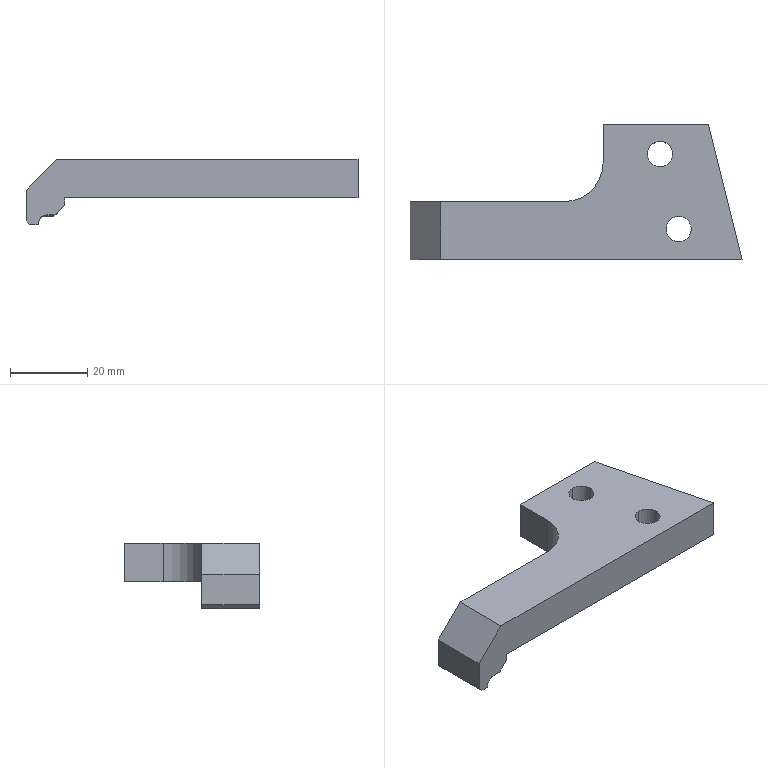Part | 1 solid | 24 faces | box 86 x 35 x 17 mm | volume 18400 mm3 | plane 13 | spline 6 | cylinder 5 | commonest cylinder face diameters 6.5 x4 20 x1
STEP:
#1=CARTESIAN_POINT('',(26.602,-12.85,-10.));
#2=VERTEX_POINT('',#1);
#3=CARTESIAN_POINT('',(26.602,-6.35,-10.));
#4=VERTEX_POINT('',#3);
#5=CARTESIAN_POINT('',(26.602,-9.6,-10.));
#6=DIRECTION('',(0.,0.,1.));
#7=DIRECTION('',(0.,1.,0.));
#8=AXIS2_PLACEMENT_3D('',#5,#6,#7);
#9=CIRCLE('',#8,3.25);
#10=EDGE_CURVE('',#2,#4,#9,.T.);
#11=ORIENTED_EDGE('',*,*,#10,.F.);
#12=CARTESIAN_POINT('',(26.602,-12.85,0.));
#13=VERTEX_POINT('',#12);
#14=CARTESIAN_POINT('',(26.602,-12.85,0.));
#15=DIRECTION('',(0.,0.,1.));
#16=VECTOR('',#15,1000.);
#17=LINE('',#14,#16);
#18=EDGE_CURVE('',#2,#13,#17,.T.);
#19=ORIENTED_EDGE('',*,*,#18,.T.);
#20=CARTESIAN_POINT('',(26.602,-6.35,0.));
#21=VERTEX_POINT('',#20);
#22=CARTESIAN_POINT('',(26.602,-9.6,0.));
#23=DIRECTION('',(0.,0.,1.));
#24=DIRECTION('',(0.,1.,0.));
#25=AXIS2_PLACEMENT_3D('',#22,#23,#24);
#26=CIRCLE('',#25,3.25);
#27=EDGE_CURVE('',#13,#21,#26,.T.);
#28=ORIENTED_EDGE('',*,*,#27,.T.);
#29=CARTESIAN_POINT('',(26.602,-6.35,0.));
#30=DIRECTION('',(0.,0.,1.));
#31=VECTOR('',#30,1000.);
#32=LINE('',#29,#31);
#33=EDGE_CURVE('',#4,#21,#32,.T.);
#34=ORIENTED_EDGE('',*,*,#33,.F.);
#35=EDGE_LOOP('',(#11,#19,#28,#34));
#36=FACE_BOUND('',#35,.T.);
#37=CARTESIAN_POINT('',(26.602,-9.6,0.));
#38=DIRECTION('',(0.,0.,1.));
#39=DIRECTION('',(0.,-1.,0.));
#40=AXIS2_PLACEMENT_3D('',#37,#38,#39);
#41=CYLINDRICAL_SURFACE('',#40,3.25);
#42=ADVANCED_FACE('',(#36),#41,.F.);
#43=CARTESIAN_POINT('',(21.763,6.556,-10.));
#44=VERTEX_POINT('',#43);
#45=CARTESIAN_POINT('',(21.763,13.056,-10.));
#46=VERTEX_POINT('',#45);
#47=CARTESIAN_POINT('',(21.763,9.806,-10.));
#48=DIRECTION('',(0.,0.,1.));
#49=DIRECTION('',(0.,1.,0.));
#50=AXIS2_PLACEMENT_3D('',#47,#48,#49);
#51=CIRCLE('',#50,3.25);
#52=EDGE_CURVE('',#44,#46,#51,.T.);
#53=ORIENTED_EDGE('',*,*,#52,.F.);
#54=CARTESIAN_POINT('',(21.763,6.556,0.));
#55=VERTEX_POINT('',#54);
#56=CARTESIAN_POINT('',(21.763,6.556,0.));
#57=DIRECTION('',(0.,0.,1.));
#58=VECTOR('',#57,1000.);
#59=LINE('',#56,#58);
#60=EDGE_CURVE('',#44,#55,#59,.T.);
#61=ORIENTED_EDGE('',*,*,#60,.T.);
#62=CARTESIAN_POINT('',(21.763,13.056,0.));
#63=VERTEX_POINT('',#62);
#64=CARTESIAN_POINT('',(21.763,9.806,0.));
#65=DIRECTION('',(0.,0.,1.));
#66=DIRECTION('',(0.,1.,0.));
#67=AXIS2_PLACEMENT_3D('',#64,#65,#66);
#68=CIRCLE('',#67,3.25);
#69=EDGE_CURVE('',#55,#63,#68,.T.);
#70=ORIENTED_EDGE('',*,*,#69,.T.);
#71=CARTESIAN_POINT('',(21.763,13.056,0.));
#72=DIRECTION('',(0.,0.,1.));
#73=VECTOR('',#72,1000.);
#74=LINE('',#71,#73);
#75=EDGE_CURVE('',#46,#63,#74,.T.);
#76=ORIENTED_EDGE('',*,*,#75,.F.);
#77=EDGE_LOOP('',(#53,#61,#70,#76));
#78=FACE_BOUND('',#77,.T.);
#79=CARTESIAN_POINT('',(21.763,9.806,0.));
#80=DIRECTION('',(0.,0.,1.));
#81=DIRECTION('',(0.,-1.,0.));
#82=AXIS2_PLACEMENT_3D('',#79,#80,#81);
#83=CYLINDRICAL_SURFACE('',#82,3.25);
#84=ADVANCED_FACE('',(#78),#83,.F.);
#85=CARTESIAN_POINT('',(21.763,9.806,0.));
#86=DIRECTION('',(0.,0.,1.));
#87=DIRECTION('',(0.,1.,0.));
#88=AXIS2_PLACEMENT_3D('',#85,#86,#87);
#89=CIRCLE('',#88,3.25);
#90=EDGE_CURVE('',#63,#55,#89,.T.);
#91=ORIENTED_EDGE('',*,*,#90,.F.);
#92=ORIENTED_EDGE('',*,*,#69,.F.);
#93=EDGE_LOOP('',(#91,#92));
#94=FACE_BOUND('',#93,.T.);
#95=CARTESIAN_POINT('',(26.602,-9.6,0.));
#96=DIRECTION('',(0.,0.,1.));
#97=DIRECTION('',(0.,1.,0.));
#98=AXIS2_PLACEMENT_3D('',#95,#96,#97);
#99=CIRCLE('',#98,3.25);
#100=EDGE_CURVE('',#21,#13,#99,.T.);
#101=ORIENTED_EDGE('',*,*,#100,.F.);
#102=ORIENTED_EDGE('',*,*,#27,.F.);
#103=EDGE_LOOP('',(#101,#102));
#104=FACE_BOUND('',#103,.T.);
#105=CARTESIAN_POINT('',(7.,17.5,0.));
#106=VERTEX_POINT('',#105);
#107=CARTESIAN_POINT('',(7.,7.5,0.));
#108=VERTEX_POINT('',#107);
#109=CARTESIAN_POINT('',(7.,17.5,0.));
#110=DIRECTION('',(0.,-1.,0.));
#111=VECTOR('',#110,1000.);
#112=LINE('',#109,#111);
#113=EDGE_CURVE('',#106,#108,#112,.T.);
#114=ORIENTED_EDGE('',*,*,#113,.T.);
#115=CARTESIAN_POINT('',(-3.,-2.5,0.));
#116=VERTEX_POINT('',#115);
#117=CARTESIAN_POINT('',(-3.,7.5,0.));
#118=DIRECTION('',(0.,0.,-1.));
#119=DIRECTION('',(-1.,0.,0.));
#120=AXIS2_PLACEMENT_3D('',#117,#118,#119);
#121=CIRCLE('',#120,10.);
#122=EDGE_CURVE('',#108,#116,#121,.T.);
#123=ORIENTED_EDGE('',*,*,#122,.T.);
#124=CARTESIAN_POINT('',(-35.,-2.5,0.));
#125=VERTEX_POINT('',#124);
#126=CARTESIAN_POINT('',(-43.,-2.5,0.));
#127=DIRECTION('',(1.,0.,0.));
#128=VECTOR('',#127,1000.);
#129=LINE('',#126,#128);
#130=EDGE_CURVE('',#125,#116,#129,.T.);
#131=ORIENTED_EDGE('',*,*,#130,.F.);
#132=CARTESIAN_POINT('',(-35.,-17.5,0.));
#133=VERTEX_POINT('',#132);
#134=CARTESIAN_POINT('',(-35.,17.5,0.));
#135=DIRECTION('',(0.,-1.,0.));
#136=VECTOR('',#135,1000.);
#137=LINE('',#134,#136);
#138=EDGE_CURVE('',#125,#133,#137,.T.);
#139=ORIENTED_EDGE('',*,*,#138,.T.);
#140=CARTESIAN_POINT('',(43.,-17.5,0.));
#141=VERTEX_POINT('',#140);
#142=CARTESIAN_POINT('',(-43.,-17.5,0.));
#143=DIRECTION('',(1.,0.,0.));
#144=VECTOR('',#143,1000.);
#145=LINE('',#142,#144);
#146=EDGE_CURVE('',#133,#141,#145,.T.);
#147=ORIENTED_EDGE('',*,*,#146,.T.);
#148=CARTESIAN_POINT('',(34.274,17.5,0.));
#149=VERTEX_POINT('',#148);
#150=CARTESIAN_POINT('',(34.274,17.5,0.));
#151=DIRECTION('',(0.2419,-0.9703,0.));
#152=VECTOR('',#151,1000.);
#153=LINE('',#150,#152);
#154=EDGE_CURVE('',#149,#141,#153,.T.);
#155=ORIENTED_EDGE('',*,*,#154,.F.);
#156=CARTESIAN_POINT('',(-43.,17.5,0.));
#157=DIRECTION('',(1.,0.,0.));
#158=VECTOR('',#157,1000.);
#159=LINE('',#156,#158);
#160=EDGE_CURVE('',#106,#149,#159,.T.);
#161=ORIENTED_EDGE('',*,*,#160,.F.);
#162=EDGE_LOOP('',(#114,#123,#131,#139,#147,#155,#161));
#163=FACE_BOUND('',#162,.T.);
#164=CARTESIAN_POINT('',(-43.,17.5,0.));
#165=DIRECTION('',(0.,0.,-1.));
#166=DIRECTION('',(1.,0.,0.));
#167=AXIS2_PLACEMENT_3D('',#164,#165,#166);
#168=PLANE('',#167);
#169=ADVANCED_FACE('',(#94,#104,#163),#168,.F.);
#170=CARTESIAN_POINT('',(21.763,9.806,-10.));
#171=DIRECTION('',(0.,0.,1.));
#172=DIRECTION('',(0.,1.,0.));
#173=AXIS2_PLACEMENT_3D('',#170,#171,#172);
#174=CIRCLE('',#173,3.25);
#175=EDGE_CURVE('',#46,#44,#174,.T.);
#176=ORIENTED_EDGE('',*,*,#175,.T.);
#177=ORIENTED_EDGE('',*,*,#52,.T.);
#178=EDGE_LOOP('',(#176,#177));
#179=FACE_BOUND('',#178,.T.);
#180=CARTESIAN_POINT('',(26.602,-9.6,-10.));
#181=DIRECTION('',(0.,0.,1.));
#182=DIRECTION('',(0.,1.,0.));
#183=AXIS2_PLACEMENT_3D('',#180,#181,#182);
#184=CIRCLE('',#183,3.25);
#185=EDGE_CURVE('',#4,#2,#184,.T.);
#186=ORIENTED_EDGE('',*,*,#185,.T.);
#187=ORIENTED_EDGE('',*,*,#10,.T.);
#188=EDGE_LOOP('',(#186,#187));
#189=FACE_BOUND('',#188,.T.);
#190=CARTESIAN_POINT('',(7.,17.5,-10.));
#191=VERTEX_POINT('',#190);
#192=CARTESIAN_POINT('',(7.,7.5,-10.));
#193=VERTEX_POINT('',#192);
#194=CARTESIAN_POINT('',(7.,17.5,-10.));
#195=DIRECTION('',(0.,-1.,0.));
#196=VECTOR('',#195,1000.);
#197=LINE('',#194,#196);
#198=EDGE_CURVE('',#191,#193,#197,.T.);
#199=ORIENTED_EDGE('',*,*,#198,.F.);
#200=CARTESIAN_POINT('',(34.274,17.5,-10.));
#201=VERTEX_POINT('',#200);
#202=CARTESIAN_POINT('',(43.,17.5,-10.));
#203=DIRECTION('',(-1.,0.,0.));
#204=VECTOR('',#203,1000.);
#205=LINE('',#202,#204);
#206=EDGE_CURVE('',#201,#191,#205,.T.);
#207=ORIENTED_EDGE('',*,*,#206,.F.);
#208=CARTESIAN_POINT('',(43.,-17.5,-10.));
#209=VERTEX_POINT('',#208);
#210=CARTESIAN_POINT('',(34.274,17.5,-10.));
#211=DIRECTION('',(-0.2419,0.9703,0.));
#212=VECTOR('',#211,1000.);
#213=LINE('',#210,#212);
#214=EDGE_CURVE('',#209,#201,#213,.T.);
#215=ORIENTED_EDGE('',*,*,#214,.F.);
#216=CARTESIAN_POINT('',(-33.,-17.5,-10.));
#217=VERTEX_POINT('',#216);
#218=CARTESIAN_POINT('',(43.,-17.5,-10.));
#219=DIRECTION('',(-1.,0.,0.));
#220=VECTOR('',#219,1000.);
#221=LINE('',#218,#220);
#222=EDGE_CURVE('',#209,#217,#221,.T.);
#223=ORIENTED_EDGE('',*,*,#222,.T.);
#224=CARTESIAN_POINT('',(-33.,-2.5,-10.));
#225=VERTEX_POINT('',#224);
#226=CARTESIAN_POINT('',(-33.,17.5,-10.));
#227=DIRECTION('',(0.,-1.,0.));
#228=VECTOR('',#227,1000.);
#229=LINE('',#226,#228);
#230=EDGE_CURVE('',#225,#217,#229,.T.);
#231=ORIENTED_EDGE('',*,*,#230,.F.);
#232=CARTESIAN_POINT('',(-3.,-2.5,-10.));
#233=VERTEX_POINT('',#232);
#234=CARTESIAN_POINT('',(43.,-2.5,-10.));
#235=DIRECTION('',(1.,0.,0.));
#236=VECTOR('',#235,1000.);
#237=LINE('',#234,#236);
#238=EDGE_CURVE('',#225,#233,#237,.T.);
#239=ORIENTED_EDGE('',*,*,#238,.T.);
#240=CARTESIAN_POINT('',(-3.,7.5,-10.));
#241=DIRECTION('',(0.,0.,1.));
#242=DIRECTION('',(0.,1.,0.));
#243=AXIS2_PLACEMENT_3D('',#240,#241,#242);
#244=CIRCLE('',#243,10.);
#245=EDGE_CURVE('',#233,#193,#244,.T.);
#246=ORIENTED_EDGE('',*,*,#245,.T.);
#247=EDGE_LOOP('',(#199,#207,#215,#223,#231,#239,#246));
#248=FACE_BOUND('',#247,.T.);
#249=CARTESIAN_POINT('',(43.,17.5,-10.));
#250=DIRECTION('',(0.,0.,1.));
#251=DIRECTION('',(0.,-1.,0.));
#252=AXIS2_PLACEMENT_3D('',#249,#250,#251);
#253=PLANE('',#252);
#254=ADVANCED_FACE('',(#179,#189,#248),#253,.F.);
#255=ORIENTED_EDGE('',*,*,#206,.T.);
#256=CARTESIAN_POINT('',(7.,17.5,-30.));
#257=DIRECTION('',(0.,0.,1.));
#258=VECTOR('',#257,1000.);
#259=LINE('',#256,#258);
#260=EDGE_CURVE('',#191,#106,#259,.T.);
#261=ORIENTED_EDGE('',*,*,#260,.T.);
#262=ORIENTED_EDGE('',*,*,#160,.T.);
#263=CARTESIAN_POINT('',(34.274,17.5,-46.071));
#264=DIRECTION('',(0.,0.,1.));
#265=VECTOR('',#264,1000.);
#266=LINE('',#263,#265);
#267=EDGE_CURVE('',#201,#149,#266,.T.);
#268=ORIENTED_EDGE('',*,*,#267,.F.);
#269=EDGE_LOOP('',(#255,#261,#262,#268));
#270=FACE_BOUND('',#269,.T.);
#271=CARTESIAN_POINT('',(43.,17.5,0.));
#272=DIRECTION('',(0.,1.,0.));
#273=DIRECTION('',(0.,0.,1.));
#274=AXIS2_PLACEMENT_3D('',#271,#272,#273);
#275=PLANE('',#274);
#276=ADVANCED_FACE('',(#270),#275,.T.);
#277=CARTESIAN_POINT('',(-33.,-17.5,-12.));
#278=VERTEX_POINT('',#277);
#279=CARTESIAN_POINT('',(-33.,-2.5,-12.));
#280=VERTEX_POINT('',#279);
#281=CARTESIAN_POINT('',(-33.,17.5,-12.));
#282=DIRECTION('',(0.,1.,0.));
#283=VECTOR('',#282,1000.);
#284=LINE('',#281,#283);
#285=EDGE_CURVE('',#278,#280,#284,.T.);
#286=ORIENTED_EDGE('',*,*,#285,.T.);
#287=CARTESIAN_POINT('',(-33.,-2.5,-10.));
#288=DIRECTION('',(0.,0.,1.));
#289=VECTOR('',#288,1000.);
#290=LINE('',#287,#289);
#291=EDGE_CURVE('',#280,#225,#290,.T.);
#292=ORIENTED_EDGE('',*,*,#291,.T.);
#293=ORIENTED_EDGE('',*,*,#230,.T.);
#294=CARTESIAN_POINT('',(-33.,-17.5,-10.));
#295=DIRECTION('',(0.,0.,-1.));
#296=VECTOR('',#295,1000.);
#297=LINE('',#294,#296);
#298=EDGE_CURVE('',#217,#278,#297,.T.);
#299=ORIENTED_EDGE('',*,*,#298,.T.);
#300=EDGE_LOOP('',(#286,#292,#293,#299));
#301=FACE_BOUND('',#300,.T.);
#302=CARTESIAN_POINT('',(-33.,17.5,-10.));
#303=DIRECTION('',(-1.,0.,0.));
#304=DIRECTION('',(0.,-1.,0.));
#305=AXIS2_PLACEMENT_3D('',#302,#303,#304);
#306=PLANE('',#305);
#307=ADVANCED_FACE('',(#301),#306,.F.);
#308=CARTESIAN_POINT('',(-39.879,-17.5,-17.));
#309=VERTEX_POINT('',#308);
#310=CARTESIAN_POINT('',(-42.,-17.5,-17.));
#311=VERTEX_POINT('',#310);
#312=CARTESIAN_POINT('',(-33.,-17.5,-17.));
#313=DIRECTION('',(-1.,0.,0.));
#314=VECTOR('',#313,1000.);
#315=LINE('',#312,#314);
#316=EDGE_CURVE('',#309,#311,#315,.T.);
#317=ORIENTED_EDGE('',*,*,#316,.T.);
#318=CARTESIAN_POINT('',(-42.,-2.5,-17.));
#319=VERTEX_POINT('',#318);
#320=CARTESIAN_POINT('',(-42.,17.5,-17.));
#321=DIRECTION('',(0.,1.,0.));
#322=VECTOR('',#321,1000.);
#323=LINE('',#320,#322);
#324=EDGE_CURVE('',#311,#319,#323,.T.);
#325=ORIENTED_EDGE('',*,*,#324,.T.);
#326=CARTESIAN_POINT('',(-40.478,-2.5,-17.));
#327=VERTEX_POINT('',#326);
#328=CARTESIAN_POINT('',(-33.,-2.5,-17.));
#329=DIRECTION('',(1.,0.,0.));
#330=VECTOR('',#329,1000.);
#331=LINE('',#328,#330);
#332=EDGE_CURVE('',#319,#327,#331,.T.);
#333=ORIENTED_EDGE('',*,*,#332,.T.);
#334=CARTESIAN_POINT('',(-40.319,-4.319,-17.));
#335=VERTEX_POINT('',#334);
#336=CARTESIAN_POINT('',(-40.478,-2.5,-17.));
#337=CARTESIAN_POINT('',(-40.423,-3.106,-17.));
#338=CARTESIAN_POINT('',(-40.37,-3.713,-17.));
#339=CARTESIAN_POINT('',(-40.319,-4.319,-17.));
#340=B_SPLINE_CURVE_WITH_KNOTS('',3,(#336,#337,#338,#339),.UNSPECIFIED.,.F.,.F.,(4,4),(0.,0.001826),.UNSPECIFIED.);
#341=EDGE_CURVE('',#327,#335,#340,.T.);
#342=ORIENTED_EDGE('',*,*,#341,.T.);
#343=CARTESIAN_POINT('',(-39.884,-12.652,-17.));
#344=VERTEX_POINT('',#343);
#345=CARTESIAN_POINT('',(-40.319,-4.319,-17.));
#346=CARTESIAN_POINT('',(-40.085,-7.091,-17.));
#347=CARTESIAN_POINT('',(-39.956,-9.871,-17.));
#348=CARTESIAN_POINT('',(-39.884,-12.652,-17.));
#349=B_SPLINE_CURVE_WITH_KNOTS('',3,(#345,#346,#347,#348),.UNSPECIFIED.,.F.,.F.,(4,4),(0.,0.008345),.UNSPECIFIED.);
#350=EDGE_CURVE('',#335,#344,#349,.T.);
#351=ORIENTED_EDGE('',*,*,#350,.T.);
#352=CARTESIAN_POINT('',(-39.884,-12.652,-17.));
#353=CARTESIAN_POINT('',(-39.842,-14.268,-17.));
#354=CARTESIAN_POINT('',(-39.855,-15.884,-17.));
#355=CARTESIAN_POINT('',(-39.879,-17.5,-17.));
#356=B_SPLINE_CURVE_WITH_KNOTS('',3,(#352,#353,#354,#355),.UNSPECIFIED.,.F.,.F.,(4,4),(0.,0.004848),.UNSPECIFIED.);
#357=EDGE_CURVE('',#344,#309,#356,.T.);
#358=ORIENTED_EDGE('',*,*,#357,.T.);
#359=EDGE_LOOP('',(#317,#325,#333,#342,#351,#358));
#360=FACE_BOUND('',#359,.T.);
#361=CARTESIAN_POINT('',(-33.,17.5,-17.));
#362=DIRECTION('',(0.,0.,1.));
#363=DIRECTION('',(-1.,0.,0.));
#364=AXIS2_PLACEMENT_3D('',#361,#362,#363);
#365=PLANE('',#364);
#366=ADVANCED_FACE('',(#360),#365,.F.);
#367=CARTESIAN_POINT('',(-43.,-2.5,-16.));
#368=VERTEX_POINT('',#367);
#369=CARTESIAN_POINT('',(-43.,-2.5,-8.));
#370=VERTEX_POINT('',#369);
#371=CARTESIAN_POINT('',(-43.,-2.5,-30.));
#372=DIRECTION('',(0.,0.,1.));
#373=VECTOR('',#372,1000.);
#374=LINE('',#371,#373);
#375=EDGE_CURVE('',#368,#370,#374,.T.);
#376=ORIENTED_EDGE('',*,*,#375,.F.);
#377=CARTESIAN_POINT('',(-43.,-17.5,-16.));
#378=VERTEX_POINT('',#377);
#379=CARTESIAN_POINT('',(-43.,17.5,-16.));
#380=DIRECTION('',(0.,-1.,0.));
#381=VECTOR('',#380,1000.);
#382=LINE('',#379,#381);
#383=EDGE_CURVE('',#368,#378,#382,.T.);
#384=ORIENTED_EDGE('',*,*,#383,.T.);
#385=CARTESIAN_POINT('',(-43.,-17.5,-8.));
#386=VERTEX_POINT('',#385);
#387=CARTESIAN_POINT('',(-43.,-17.5,-17.));
#388=DIRECTION('',(0.,0.,1.));
#389=VECTOR('',#388,1000.);
#390=LINE('',#387,#389);
#391=EDGE_CURVE('',#378,#386,#390,.T.);
#392=ORIENTED_EDGE('',*,*,#391,.T.);
#393=CARTESIAN_POINT('',(-43.,17.5,-8.));
#394=DIRECTION('',(0.,1.,0.));
#395=VECTOR('',#394,1000.);
#396=LINE('',#393,#395);
#397=EDGE_CURVE('',#386,#370,#396,.T.);
#398=ORIENTED_EDGE('',*,*,#397,.T.);
#399=EDGE_LOOP('',(#376,#384,#392,#398));
#400=FACE_BOUND('',#399,.T.);
#401=CARTESIAN_POINT('',(-43.,17.5,-17.));
#402=DIRECTION('',(1.,0.,0.));
#403=DIRECTION('',(0.,1.,0.));
#404=AXIS2_PLACEMENT_3D('',#401,#402,#403);
#405=PLANE('',#404);
#406=ADVANCED_FACE('',(#400),#405,.F.);
#407=ORIENTED_EDGE('',*,*,#391,.F.);
#408=CARTESIAN_POINT('',(-43.,-17.5,-16.));
#409=DIRECTION('',(0.7071,0.,-0.7071));
#410=VECTOR('',#409,1000.);
#411=LINE('',#408,#410);
#412=EDGE_CURVE('',#378,#311,#411,.T.);
#413=ORIENTED_EDGE('',*,*,#412,.T.);
#414=ORIENTED_EDGE('',*,*,#316,.F.);
#415=CARTESIAN_POINT('',(-38.523,-17.5,-14.597));
#416=VERTEX_POINT('',#415);
#417=CARTESIAN_POINT('',(-39.879,-17.5,-17.));
#418=CARTESIAN_POINT('',(-39.871,-17.5,-16.507));
#419=CARTESIAN_POINT('',(-39.78,-17.5,-15.474));
#420=CARTESIAN_POINT('',(-38.973,-17.5,-14.805));
#421=CARTESIAN_POINT('',(-38.523,-17.5,-14.597));
#422=B_SPLINE_CURVE_WITH_KNOTS('',3,(#417,#418,#419,#420,#421),.UNSPECIFIED.,.F.,.F.,(4,1,4),(0.,0.001474,0.002948),.UNSPECIFIED.);
#423=EDGE_CURVE('',#309,#416,#422,.T.);
#424=ORIENTED_EDGE('',*,*,#423,.T.);
#425=CARTESIAN_POINT('',(-35.453,-17.5,-14.453));
#426=VERTEX_POINT('',#425);
#427=CARTESIAN_POINT('',(-38.523,-17.5,-14.597));
#428=CARTESIAN_POINT('',(-38.286,-17.5,-14.488));
#429=CARTESIAN_POINT('',(-37.768,-17.5,-14.429));
#430=CARTESIAN_POINT('',(-36.742,-17.5,-14.384));
#431=CARTESIAN_POINT('',(-35.968,-17.5,-14.426));
#432=CARTESIAN_POINT('',(-35.453,-17.5,-14.453));
#433=B_SPLINE_CURVE_WITH_KNOTS('',3,(#427,#428,#429,#430,#431,#432),.UNSPECIFIED.,.F.,.F.,(4,1,1,4),(0.,0.0007709,0.001542,0.003084),.UNSPECIFIED.);
#434=EDGE_CURVE('',#416,#426,#433,.T.);
#435=ORIENTED_EDGE('',*,*,#434,.T.);
#436=CARTESIAN_POINT('',(-38.,-17.5,-17.));
#437=DIRECTION('',(0.7071,0.,0.7071));
#438=VECTOR('',#437,1000.);
#439=LINE('',#436,#438);
#440=EDGE_CURVE('',#426,#278,#439,.T.);
#441=ORIENTED_EDGE('',*,*,#440,.T.);
#442=ORIENTED_EDGE('',*,*,#298,.F.);
#443=ORIENTED_EDGE('',*,*,#222,.F.);
#444=CARTESIAN_POINT('',(43.,-17.5,0.));
#445=DIRECTION('',(0.,0.,-1.));
#446=VECTOR('',#445,1000.);
#447=LINE('',#444,#446);
#448=EDGE_CURVE('',#141,#209,#447,.T.);
#449=ORIENTED_EDGE('',*,*,#448,.F.);
#450=ORIENTED_EDGE('',*,*,#146,.F.);
#451=CARTESIAN_POINT('',(-35.,-17.5,0.));
#452=DIRECTION('',(-0.7071,0.,-0.7071));
#453=VECTOR('',#452,1000.);
#454=LINE('',#451,#453);
#455=EDGE_CURVE('',#133,#386,#454,.T.);
#456=ORIENTED_EDGE('',*,*,#455,.T.);
#457=EDGE_LOOP('',(#407,#413,#414,#424,#435,#441,#442,#443,#449,#450,#456));
#458=FACE_BOUND('',#457,.T.);
#459=CARTESIAN_POINT('',(43.,-17.5,0.));
#460=DIRECTION('',(0.,1.,0.));
#461=DIRECTION('',(0.,0.,1.));
#462=AXIS2_PLACEMENT_3D('',#459,#460,#461);
#463=PLANE('',#462);
#464=ADVANCED_FACE('',(#458),#463,.F.);
#465=ORIENTED_EDGE('',*,*,#214,.T.);
#466=ORIENTED_EDGE('',*,*,#267,.T.);
#467=ORIENTED_EDGE('',*,*,#154,.T.);
#468=ORIENTED_EDGE('',*,*,#448,.T.);
#469=EDGE_LOOP('',(#465,#466,#467,#468));
#470=FACE_BOUND('',#469,.T.);
#471=CARTESIAN_POINT('',(34.274,17.5,-46.071));
#472=DIRECTION('',(-0.9703,-0.2419,0.));
#473=DIRECTION('',(0.2419,-0.9703,0.));
#474=AXIS2_PLACEMENT_3D('',#471,#472,#473);
#475=PLANE('',#474);
#476=ADVANCED_FACE('',(#470),#475,.F.);
#477=ORIENTED_EDGE('',*,*,#60,.F.);
#478=ORIENTED_EDGE('',*,*,#175,.F.);
#479=ORIENTED_EDGE('',*,*,#75,.T.);
#480=ORIENTED_EDGE('',*,*,#90,.T.);
#481=EDGE_LOOP('',(#477,#478,#479,#480));
#482=FACE_BOUND('',#481,.T.);
#483=CARTESIAN_POINT('',(21.763,9.806,0.));
#484=DIRECTION('',(0.,0.,1.));
#485=DIRECTION('',(0.,-1.,0.));
#486=AXIS2_PLACEMENT_3D('',#483,#484,#485);
#487=CYLINDRICAL_SURFACE('',#486,3.25);
#488=ADVANCED_FACE('',(#482),#487,.F.);
#489=ORIENTED_EDGE('',*,*,#18,.F.);
#490=ORIENTED_EDGE('',*,*,#185,.F.);
#491=ORIENTED_EDGE('',*,*,#33,.T.);
#492=ORIENTED_EDGE('',*,*,#100,.T.);
#493=EDGE_LOOP('',(#489,#490,#491,#492));
#494=FACE_BOUND('',#493,.T.);
#495=CARTESIAN_POINT('',(26.602,-9.6,0.));
#496=DIRECTION('',(0.,0.,1.));
#497=DIRECTION('',(0.,-1.,0.));
#498=AXIS2_PLACEMENT_3D('',#495,#496,#497);
#499=CYLINDRICAL_SURFACE('',#498,3.25);
#500=ADVANCED_FACE('',(#494),#499,.F.);
#501=CARTESIAN_POINT('',(-35.,-2.5,0.));
#502=DIRECTION('',(0.7071,0.,0.7071));
#503=VECTOR('',#502,1000.);
#504=LINE('',#501,#503);
#505=EDGE_CURVE('',#370,#125,#504,.T.);
#506=ORIENTED_EDGE('',*,*,#505,.F.);
#507=ORIENTED_EDGE('',*,*,#397,.F.);
#508=ORIENTED_EDGE('',*,*,#455,.F.);
#509=ORIENTED_EDGE('',*,*,#138,.F.);
#510=EDGE_LOOP('',(#506,#507,#508,#509));
#511=FACE_BOUND('',#510,.T.);
#512=CARTESIAN_POINT('',(-35.,17.5,0.));
#513=DIRECTION('',(0.7071,0.,-0.7071));
#514=DIRECTION('',(0.,1.,0.));
#515=AXIS2_PLACEMENT_3D('',#512,#513,#514);
#516=PLANE('',#515);
#517=ADVANCED_FACE('',(#511),#516,.F.);
#518=CARTESIAN_POINT('',(-35.6,-11.965,-14.6));
#519=VERTEX_POINT('',#518);
#520=CARTESIAN_POINT('',(-35.6,-11.965,-14.6));
#521=CARTESIAN_POINT('',(-35.556,-13.81,-14.556));
#522=CARTESIAN_POINT('',(-35.51,-15.655,-14.51));
#523=CARTESIAN_POINT('',(-35.453,-17.5,-14.453));
#524=B_SPLINE_CURVE_WITH_KNOTS('',3,(#520,#521,#522,#523),.UNSPECIFIED.,.F.,.F.,(4,4),(0.,0.005539),.UNSPECIFIED.);
#525=EDGE_CURVE('',#519,#426,#524,.T.);
#526=ORIENTED_EDGE('',*,*,#525,.F.);
#527=CARTESIAN_POINT('',(-35.775,-3.519,-14.775));
#528=VERTEX_POINT('',#527);
#529=CARTESIAN_POINT('',(-35.775,-3.519,-14.775));
#530=CARTESIAN_POINT('',(-35.716,-6.334,-14.716));
#531=CARTESIAN_POINT('',(-35.667,-9.15,-14.667));
#532=CARTESIAN_POINT('',(-35.6,-11.965,-14.6));
#533=B_SPLINE_CURVE_WITH_KNOTS('',3,(#529,#530,#531,#532),.UNSPECIFIED.,.F.,.F.,(4,4),(0.,0.008449),.UNSPECIFIED.);
#534=EDGE_CURVE('',#528,#519,#533,.T.);
#535=ORIENTED_EDGE('',*,*,#534,.F.);
#536=CARTESIAN_POINT('',(-35.797,-2.5,-14.797));
#537=VERTEX_POINT('',#536);
#538=CARTESIAN_POINT('',(-35.797,-2.5,-14.797));
#539=CARTESIAN_POINT('',(-35.789,-2.84,-14.789));
#540=CARTESIAN_POINT('',(-35.782,-3.179,-14.782));
#541=CARTESIAN_POINT('',(-35.775,-3.519,-14.775));
#542=B_SPLINE_CURVE_WITH_KNOTS('',3,(#538,#539,#540,#541),.UNSPECIFIED.,.F.,.F.,(4,4),(0.,0.00102),.UNSPECIFIED.);
#543=EDGE_CURVE('',#537,#528,#542,.T.);
#544=ORIENTED_EDGE('',*,*,#543,.F.);
#545=CARTESIAN_POINT('',(-38.,-2.5,-17.));
#546=DIRECTION('',(-0.7071,0.,-0.7071));
#547=VECTOR('',#546,1000.);
#548=LINE('',#545,#547);
#549=EDGE_CURVE('',#280,#537,#548,.T.);
#550=ORIENTED_EDGE('',*,*,#549,.F.);
#551=ORIENTED_EDGE('',*,*,#285,.F.);
#552=ORIENTED_EDGE('',*,*,#440,.F.);
#553=EDGE_LOOP('',(#526,#535,#544,#550,#551,#552));
#554=FACE_BOUND('',#553,.T.);
#555=CARTESIAN_POINT('',(-38.,17.5,-17.));
#556=DIRECTION('',(-0.7071,0.,0.7071));
#557=DIRECTION('',(0.,1.,0.));
#558=AXIS2_PLACEMENT_3D('',#555,#556,#557);
#559=PLANE('',#558);
#560=ADVANCED_FACE('',(#554),#559,.F.);
#561=ORIENTED_EDGE('',*,*,#198,.T.);
#562=CARTESIAN_POINT('',(7.,7.5,-30.));
#563=DIRECTION('',(0.,0.,1.));
#564=VECTOR('',#563,1000.);
#565=LINE('',#562,#564);
#566=EDGE_CURVE('',#193,#108,#565,.T.);
#567=ORIENTED_EDGE('',*,*,#566,.T.);
#568=ORIENTED_EDGE('',*,*,#113,.F.);
#569=ORIENTED_EDGE('',*,*,#260,.F.);
#570=EDGE_LOOP('',(#561,#567,#568,#569));
#571=FACE_BOUND('',#570,.T.);
#572=CARTESIAN_POINT('',(7.,17.5,-30.));
#573=DIRECTION('',(-1.,0.,0.));
#574=DIRECTION('',(0.,0.,-1.));
#575=AXIS2_PLACEMENT_3D('',#572,#573,#574);
#576=PLANE('',#575);
#577=ADVANCED_FACE('',(#571),#576,.T.);
#578=ORIENTED_EDGE('',*,*,#332,.F.);
#579=CARTESIAN_POINT('',(-43.,-2.5,-16.));
#580=DIRECTION('',(-0.7071,0.,0.7071));
#581=VECTOR('',#580,1000.);
#582=LINE('',#579,#581);
#583=EDGE_CURVE('',#319,#368,#582,.T.);
#584=ORIENTED_EDGE('',*,*,#583,.T.);
#585=ORIENTED_EDGE('',*,*,#375,.T.);
#586=ORIENTED_EDGE('',*,*,#505,.T.);
#587=ORIENTED_EDGE('',*,*,#130,.T.);
#588=CARTESIAN_POINT('',(-3.,-2.5,-30.));
#589=DIRECTION('',(0.,0.,-1.));
#590=VECTOR('',#589,1000.);
#591=LINE('',#588,#590);
#592=EDGE_CURVE('',#116,#233,#591,.T.);
#593=ORIENTED_EDGE('',*,*,#592,.T.);
#594=ORIENTED_EDGE('',*,*,#238,.F.);
#595=ORIENTED_EDGE('',*,*,#291,.F.);
#596=ORIENTED_EDGE('',*,*,#549,.T.);
#597=CARTESIAN_POINT('',(-39.03,-2.5,-14.884));
#598=VERTEX_POINT('',#597);
#599=CARTESIAN_POINT('',(-35.797,-2.5,-14.797));
#600=CARTESIAN_POINT('',(-36.338,-2.5,-14.763));
#601=CARTESIAN_POINT('',(-37.151,-2.5,-14.728));
#602=CARTESIAN_POINT('',(-38.228,-2.5,-14.744));
#603=CARTESIAN_POINT('',(-38.777,-2.5,-14.782));
#604=CARTESIAN_POINT('',(-39.03,-2.5,-14.884));
#605=B_SPLINE_CURVE_WITH_KNOTS('',3,(#599,#600,#601,#602,#603,#604),.UNSPECIFIED.,.F.,.F.,(4,1,1,4),(0.,0.001624,0.002436,0.003248),.UNSPECIFIED.);
#606=EDGE_CURVE('',#537,#598,#605,.T.);
#607=ORIENTED_EDGE('',*,*,#606,.T.);
#608=CARTESIAN_POINT('',(-39.03,-2.5,-14.884));
#609=CARTESIAN_POINT('',(-39.455,-2.5,-15.055));
#610=CARTESIAN_POINT('',(-40.263,-2.5,-15.587));
#611=CARTESIAN_POINT('',(-40.44,-2.5,-16.543));
#612=CARTESIAN_POINT('',(-40.478,-2.5,-17.));
#613=B_SPLINE_CURVE_WITH_KNOTS('',3,(#608,#609,#610,#611,#612),.UNSPECIFIED.,.F.,.F.,(4,1,4),(0.,0.001361,0.002721),.UNSPECIFIED.);
#614=EDGE_CURVE('',#598,#327,#613,.T.);
#615=ORIENTED_EDGE('',*,*,#614,.T.);
#616=EDGE_LOOP('',(#578,#584,#585,#586,#587,#593,#594,#595,#596,#607,#615));
#617=FACE_BOUND('',#616,.T.);
#618=CARTESIAN_POINT('',(-43.,-2.5,-30.));
#619=DIRECTION('',(0.,-1.,0.));
#620=DIRECTION('',(1.,0.,0.));
#621=AXIS2_PLACEMENT_3D('',#618,#619,#620);
#622=PLANE('',#621);
#623=ADVANCED_FACE('',(#617),#622,.F.);
#624=ORIENTED_EDGE('',*,*,#245,.F.);
#625=ORIENTED_EDGE('',*,*,#592,.F.);
#626=ORIENTED_EDGE('',*,*,#122,.F.);
#627=ORIENTED_EDGE('',*,*,#566,.F.);
#628=EDGE_LOOP('',(#624,#625,#626,#627));
#629=FACE_BOUND('',#628,.T.);
#630=CARTESIAN_POINT('',(-3.,7.5,-30.));
#631=DIRECTION('',(0.,0.,1.));
#632=DIRECTION('',(-1.,0.,0.));
#633=AXIS2_PLACEMENT_3D('',#630,#631,#632);
#634=CYLINDRICAL_SURFACE('',#633,10.);
#635=ADVANCED_FACE('',(#629),#634,.F.);
#636=CARTESIAN_POINT('',(-38.887,-4.107,-14.858));
#637=VERTEX_POINT('',#636);
#638=CARTESIAN_POINT('',(-40.319,-4.319,-17.));
#639=CARTESIAN_POINT('',(-40.303,-4.31,-16.78));
#640=CARTESIAN_POINT('',(-40.25,-4.289,-16.322));
#641=CARTESIAN_POINT('',(-40.009,-4.246,-15.672));
#642=CARTESIAN_POINT('',(-39.521,-4.185,-15.162));
#643=CARTESIAN_POINT('',(-39.093,-4.136,-14.943));
#644=CARTESIAN_POINT('',(-38.887,-4.107,-14.858));
#645=B_SPLINE_CURVE_WITH_KNOTS('',3,(#638,#639,#640,#641,#642,#643,#644),.UNSPECIFIED.,.F.,.F.,(4,1,1,1,4),(0.,0.2345,0.4897,0.7448,1.),.UNSPECIFIED.);
#646=EDGE_CURVE('',#335,#637,#645,.T.);
#647=ORIENTED_EDGE('',*,*,#646,.T.);
#648=CARTESIAN_POINT('',(-38.452,-12.428,-14.711));
#649=VERTEX_POINT('',#648);
#650=CARTESIAN_POINT('',(-38.887,-4.107,-14.858));
#651=CARTESIAN_POINT('',(-38.868,-4.338,-14.854));
#652=CARTESIAN_POINT('',(-38.831,-4.799,-14.845));
#653=CARTESIAN_POINT('',(-38.777,-5.491,-14.835));
#654=CARTESIAN_POINT('',(-38.728,-6.184,-14.825));
#655=CARTESIAN_POINT('',(-38.682,-6.877,-14.817));
#656=CARTESIAN_POINT('',(-38.64,-7.57,-14.807));
#657=CARTESIAN_POINT('',(-38.602,-8.264,-14.796));
#658=CARTESIAN_POINT('',(-38.568,-8.958,-14.784));
#659=CARTESIAN_POINT('',(-38.537,-9.651,-14.771));
#660=CARTESIAN_POINT('',(-38.51,-10.345,-14.756));
#661=CARTESIAN_POINT('',(-38.487,-11.039,-14.74));
#662=CARTESIAN_POINT('',(-38.467,-11.733,-14.725));
#663=CARTESIAN_POINT('',(-38.456,-12.196,-14.714));
#664=CARTESIAN_POINT('',(-38.452,-12.428,-14.711));
#665=B_SPLINE_CURVE_WITH_KNOTS('',3,(#650,#651,#652,#653,#654,#655,#656,#657,#658,#659,#660,#661,#662,#663,#664),.UNSPECIFIED.,.F.,.F.,(4,1,1,1,1,1,1,1,1,1,1,1,4),(0.,0.08333,0.1667,0.25,0.3333,0.4167,0.5,0.5833,0.6667,0.75,0.8333,0.9167,1.),.QUASI_UNIFORM_KNOTS.);
#666=EDGE_CURVE('',#637,#649,#665,.T.);
#667=ORIENTED_EDGE('',*,*,#666,.T.);
#668=CARTESIAN_POINT('',(-38.452,-12.428,-14.711));
#669=CARTESIAN_POINT('',(-38.657,-12.451,-14.796));
#670=CARTESIAN_POINT('',(-39.086,-12.484,-15.016));
#671=CARTESIAN_POINT('',(-39.568,-12.537,-15.531));
#672=CARTESIAN_POINT('',(-39.814,-12.592,-16.198));
#673=CARTESIAN_POINT('',(-39.868,-12.63,-16.704));
#674=CARTESIAN_POINT('',(-39.882,-12.65,-16.971));
#675=CARTESIAN_POINT('',(-39.884,-12.652,-17.));
#676=B_SPLINE_CURVE_WITH_KNOTS('',3,(#668,#669,#670,#671,#672,#673,#674,#675),.UNSPECIFIED.,.F.,.F.,(4,1,1,1,1,4),(0.,0.2427,0.4854,0.7281,0.9709,1.),.UNSPECIFIED.);
#677=EDGE_CURVE('',#649,#344,#676,.T.);
#678=ORIENTED_EDGE('',*,*,#677,.T.);
#679=ORIENTED_EDGE('',*,*,#350,.F.);
#680=EDGE_LOOP('',(#647,#667,#678,#679));
#681=FACE_BOUND('',#680,.T.);
#682=CARTESIAN_POINT('',(-38.452,-12.428,-14.711));
#683=CARTESIAN_POINT('',(-38.657,-12.451,-14.796));
#684=CARTESIAN_POINT('',(-39.086,-12.484,-15.016));
#685=CARTESIAN_POINT('',(-39.568,-12.537,-15.531));
#686=CARTESIAN_POINT('',(-39.814,-12.592,-16.198));
#687=CARTESIAN_POINT('',(-39.869,-12.63,-16.71));
#688=CARTESIAN_POINT('',(-39.883,-12.651,-16.983));
#689=CARTESIAN_POINT('',(-39.885,-12.653,-17.018));
#690=CARTESIAN_POINT('',(-38.456,-12.196,-14.714));
#691=CARTESIAN_POINT('',(-38.662,-12.219,-14.8));
#692=CARTESIAN_POINT('',(-39.09,-12.252,-15.021));
#693=CARTESIAN_POINT('',(-39.573,-12.305,-15.535));
#694=CARTESIAN_POINT('',(-39.82,-12.359,-16.202));
#695=CARTESIAN_POINT('',(-39.875,-12.397,-16.714));
#696=CARTESIAN_POINT('',(-39.889,-12.417,-16.987));
#697=CARTESIAN_POINT('',(-39.891,-12.42,-17.021));
#698=CARTESIAN_POINT('',(-38.467,-11.733,-14.725));
#699=CARTESIAN_POINT('',(-38.673,-11.757,-14.81));
#700=CARTESIAN_POINT('',(-39.101,-11.791,-15.031));
#701=CARTESIAN_POINT('',(-39.585,-11.843,-15.544));
#702=CARTESIAN_POINT('',(-39.835,-11.897,-16.21));
#703=CARTESIAN_POINT('',(-39.889,-11.934,-16.722));
#704=CARTESIAN_POINT('',(-39.903,-11.953,-16.995));
#705=CARTESIAN_POINT('',(-39.905,-11.956,-17.03));
#706=CARTESIAN_POINT('',(-38.487,-11.039,-14.74));
#707=CARTESIAN_POINT('',(-38.693,-11.064,-14.826));
#708=CARTESIAN_POINT('',(-39.121,-11.098,-15.048));
#709=CARTESIAN_POINT('',(-39.607,-11.151,-15.559));
#710=CARTESIAN_POINT('',(-39.857,-11.204,-16.225));
#711=CARTESIAN_POINT('',(-39.912,-11.239,-16.736));
#712=CARTESIAN_POINT('',(-39.927,-11.258,-17.01));
#713=CARTESIAN_POINT('',(-39.929,-11.26,-17.044));
#714=CARTESIAN_POINT('',(-38.51,-10.345,-14.756));
#715=CARTESIAN_POINT('',(-38.717,-10.37,-14.841));
#716=CARTESIAN_POINT('',(-39.144,-10.406,-15.063));
#717=CARTESIAN_POINT('',(-39.629,-10.459,-15.575));
#718=CARTESIAN_POINT('',(-39.881,-10.511,-16.24));
#719=CARTESIAN_POINT('',(-39.938,-10.545,-16.752));
#720=CARTESIAN_POINT('',(-39.953,-10.563,-17.025));
#721=CARTESIAN_POINT('',(-39.955,-10.565,-17.06));
#722=CARTESIAN_POINT('',(-38.537,-9.651,-14.771));
#723=CARTESIAN_POINT('',(-38.744,-9.677,-14.855));
#724=CARTESIAN_POINT('',(-39.173,-9.713,-15.076));
#725=CARTESIAN_POINT('',(-39.657,-9.767,-15.588));
#726=CARTESIAN_POINT('',(-39.909,-9.817,-16.254));
#727=CARTESIAN_POINT('',(-39.966,-9.85,-16.766));
#728=CARTESIAN_POINT('',(-39.982,-9.868,-17.039));
#729=CARTESIAN_POINT('',(-39.984,-9.87,-17.074));
#730=CARTESIAN_POINT('',(-38.568,-8.958,-14.784));
#731=CARTESIAN_POINT('',(-38.775,-8.983,-14.868));
#732=CARTESIAN_POINT('',(-39.203,-9.021,-15.09));
#733=CARTESIAN_POINT('',(-39.687,-9.075,-15.602));
#734=CARTESIAN_POINT('',(-39.94,-9.124,-16.268));
#735=CARTESIAN_POINT('',(-39.998,-9.156,-16.78));
#736=CARTESIAN_POINT('',(-40.014,-9.172,-17.053));
#737=CARTESIAN_POINT('',(-40.016,-9.175,-17.087));
#738=CARTESIAN_POINT('',(-38.602,-8.264,-14.796));
#739=CARTESIAN_POINT('',(-38.81,-8.29,-14.88));
#740=CARTESIAN_POINT('',(-39.235,-8.329,-15.103));
#741=CARTESIAN_POINT('',(-39.717,-8.384,-15.618));
#742=CARTESIAN_POINT('',(-39.974,-8.431,-16.282));
#743=CARTESIAN_POINT('',(-40.033,-8.462,-16.794));
#744=CARTESIAN_POINT('',(-40.049,-8.478,-17.067));
#745=CARTESIAN_POINT('',(-40.05,-8.48,-17.101));
#746=CARTESIAN_POINT('',(-38.64,-7.57,-14.807));
#747=CARTESIAN_POINT('',(-38.848,-7.597,-14.89));
#748=CARTESIAN_POINT('',(-39.274,-7.638,-15.11));
#749=CARTESIAN_POINT('',(-39.754,-7.693,-15.627));
#750=CARTESIAN_POINT('',(-40.011,-7.739,-16.293));
#751=CARTESIAN_POINT('',(-40.07,-7.769,-16.804));
#752=CARTESIAN_POINT('',(-40.086,-7.785,-17.077));
#753=CARTESIAN_POINT('',(-40.088,-7.786,-17.112));
#754=CARTESIAN_POINT('',(-38.682,-6.877,-14.817));
#755=CARTESIAN_POINT('',(-38.89,-6.905,-14.9));
#756=CARTESIAN_POINT('',(-39.32,-6.947,-15.115));
#757=CARTESIAN_POINT('',(-39.805,-7.002,-15.628));
#758=CARTESIAN_POINT('',(-40.053,-7.047,-16.296));
#759=CARTESIAN_POINT('',(-40.111,-7.076,-16.809));
#760=CARTESIAN_POINT('',(-40.127,-7.091,-17.082));
#761=CARTESIAN_POINT('',(-40.128,-7.093,-17.117));
#762=CARTESIAN_POINT('',(-38.728,-6.184,-14.825));
#763=CARTESIAN_POINT('',(-38.935,-6.212,-14.909));
#764=CARTESIAN_POINT('',(-39.367,-6.256,-15.122));
#765=CARTESIAN_POINT('',(-39.852,-6.312,-15.634));
#766=CARTESIAN_POINT('',(-40.098,-6.356,-16.303));
#767=CARTESIAN_POINT('',(-40.154,-6.384,-16.817));
#768=CARTESIAN_POINT('',(-40.17,-6.398,-17.09));
#769=CARTESIAN_POINT('',(-40.172,-6.4,-17.125));
#770=CARTESIAN_POINT('',(-38.777,-5.491,-14.835));
#771=CARTESIAN_POINT('',(-38.985,-5.52,-14.918));
#772=CARTESIAN_POINT('',(-39.413,-5.565,-15.135));
#773=CARTESIAN_POINT('',(-39.896,-5.623,-15.65));
#774=CARTESIAN_POINT('',(-40.144,-5.667,-16.318));
#775=CARTESIAN_POINT('',(-40.201,-5.693,-16.831));
#776=CARTESIAN_POINT('',(-40.217,-5.707,-17.104));
#777=CARTESIAN_POINT('',(-40.219,-5.708,-17.139));
#778=CARTESIAN_POINT('',(-38.831,-4.799,-14.845));
#779=CARTESIAN_POINT('',(-39.037,-4.828,-14.929));
#780=CARTESIAN_POINT('',(-39.463,-4.875,-15.15));
#781=CARTESIAN_POINT('',(-39.946,-4.934,-15.665));
#782=CARTESIAN_POINT('',(-40.196,-4.979,-16.332));
#783=CARTESIAN_POINT('',(-40.253,-5.003,-16.845));
#784=CARTESIAN_POINT('',(-40.27,-5.016,-17.118));
#785=CARTESIAN_POINT('',(-40.272,-5.017,-17.153));
#786=CARTESIAN_POINT('',(-38.868,-4.338,-14.854));
#787=CARTESIAN_POINT('',(-39.074,-4.367,-14.938));
#788=CARTESIAN_POINT('',(-39.501,-4.415,-15.158));
#789=CARTESIAN_POINT('',(-39.988,-4.476,-15.67));
#790=CARTESIAN_POINT('',(-40.236,-4.52,-16.337));
#791=CARTESIAN_POINT('',(-40.291,-4.543,-16.85));
#792=CARTESIAN_POINT('',(-40.308,-4.555,-17.124));
#793=CARTESIAN_POINT('',(-40.31,-4.556,-17.158));
#794=CARTESIAN_POINT('',(-38.887,-4.107,-14.858));
#795=CARTESIAN_POINT('',(-39.093,-4.136,-14.943));
#796=CARTESIAN_POINT('',(-39.521,-4.185,-15.162));
#797=CARTESIAN_POINT('',(-40.009,-4.246,-15.672));
#798=CARTESIAN_POINT('',(-40.256,-4.29,-16.34));
#799=CARTESIAN_POINT('',(-40.311,-4.313,-16.853));
#800=CARTESIAN_POINT('',(-40.328,-4.324,-17.127));
#801=CARTESIAN_POINT('',(-40.329,-4.326,-17.162));
#802=B_SPLINE_SURFACE_WITH_KNOTS('',3,3,((#682,#683,#684,#685,#686,#687,#688,#689),(#690,#691,#692,#693,#694,#695,#696,#697),(#698,#699,#700,#701,#702,#703,#704,#705),(#706,#707,#708,#709,#710,#711,#712,#713),(#714,#715,#716,#717,#718,#719,#720,#721),(#722,#723,#724,#725,#726,#727,#728,#729),(#730,#731,#732,#733,#734,#735,#736,#737),(#738,#739,#740,#741,#742,#743,#744,#745),(#746,#747,#748,#749,#750,#751,#752,#753),(#754,#755,#756,#757,#758,#759,#760,#761),(#762,#763,#764,#765,#766,#767,#768,#769),(#770,#771,#772,#773,#774,#775,#776,#777),(#778,#779,#780,#781,#782,#783,#784,#785),(#786,#787,#788,#789,#790,#791,#792,#793),(#794,#795,#796,#797,#798,#799,#800,#801)),.UNSPECIFIED.,.F.,.F.,.F.,(4,1,1,1,1,1,1,1,1,1,1,1,4),(4,1,1,1,1,4),(0.,0.08333,0.1667,0.25,0.3333,0.4167,0.5,0.5833,0.6667,0.75,0.8333,0.9167,1.),(0.,0.08333,0.1667,0.25,0.3333,0.3454),.UNSPECIFIED.);
#803=ADVANCED_FACE('',(#681),#802,.F.);
#804=ORIENTED_EDGE('',*,*,#677,.F.);
#805=CARTESIAN_POINT('',(-38.523,-17.5,-14.597));
#806=CARTESIAN_POINT('',(-38.509,-17.2,-14.602));
#807=CARTESIAN_POINT('',(-38.477,-16.437,-14.617));
#808=CARTESIAN_POINT('',(-38.442,-15.21,-14.647));
#809=CARTESIAN_POINT('',(-38.432,-14.051,-14.68));
#810=CARTESIAN_POINT('',(-38.439,-13.123,-14.7));
#811=CARTESIAN_POINT('',(-38.447,-12.659,-14.707));
#812=CARTESIAN_POINT('',(-38.452,-12.428,-14.711));
#813=B_SPLINE_CURVE_WITH_KNOTS('',3,(#805,#806,#807,#808,#809,#810,#811,#812),.UNSPECIFIED.,.F.,.F.,(4,1,1,1,1,4),(0.,0.1774,0.4516,0.7258,0.8629,1.),.UNSPECIFIED.);
#814=EDGE_CURVE('',#416,#649,#813,.T.);
#815=ORIENTED_EDGE('',*,*,#814,.F.);
#816=ORIENTED_EDGE('',*,*,#423,.F.);
#817=ORIENTED_EDGE('',*,*,#357,.F.);
#818=EDGE_LOOP('',(#804,#815,#816,#817));
#819=FACE_BOUND('',#818,.T.);
#820=CARTESIAN_POINT('',(-39.884,-17.868,-17.018));
#821=CARTESIAN_POINT('',(-39.883,-17.787,-17.018));
#822=CARTESIAN_POINT('',(-39.879,-17.469,-17.018));
#823=CARTESIAN_POINT('',(-39.87,-16.913,-17.019));
#824=CARTESIAN_POINT('',(-39.861,-16.202,-17.02));
#825=CARTESIAN_POINT('',(-39.855,-15.49,-17.026));
#826=CARTESIAN_POINT('',(-39.853,-14.78,-17.039));
#827=CARTESIAN_POINT('',(-39.858,-14.072,-17.051));
#828=CARTESIAN_POINT('',(-39.869,-13.364,-17.061));
#829=CARTESIAN_POINT('',(-39.881,-12.892,-17.068));
#830=CARTESIAN_POINT('',(-39.887,-12.657,-17.072));
#831=CARTESIAN_POINT('',(-39.884,-17.863,-16.965));
#832=CARTESIAN_POINT('',(-39.883,-17.782,-16.965));
#833=CARTESIAN_POINT('',(-39.878,-17.464,-16.965));
#834=CARTESIAN_POINT('',(-39.87,-16.908,-16.966));
#835=CARTESIAN_POINT('',(-39.86,-16.197,-16.967));
#836=CARTESIAN_POINT('',(-39.853,-15.486,-16.974));
#837=CARTESIAN_POINT('',(-39.851,-14.776,-16.987));
#838=CARTESIAN_POINT('',(-39.856,-14.068,-16.999));
#839=CARTESIAN_POINT('',(-39.867,-13.36,-17.008));
#840=CARTESIAN_POINT('',(-39.879,-12.888,-17.015));
#841=CARTESIAN_POINT('',(-39.885,-12.653,-17.019));
#842=CARTESIAN_POINT('',(-39.877,-17.835,-16.674));
#843=CARTESIAN_POINT('',(-39.876,-17.755,-16.674));
#844=CARTESIAN_POINT('',(-39.871,-17.437,-16.674));
#845=CARTESIAN_POINT('',(-39.862,-16.882,-16.674));
#846=CARTESIAN_POINT('',(-39.851,-16.171,-16.675));
#847=CARTESIAN_POINT('',(-39.842,-15.461,-16.682));
#848=CARTESIAN_POINT('',(-39.838,-14.751,-16.695));
#849=CARTESIAN_POINT('',(-39.842,-14.044,-16.707));
#850=CARTESIAN_POINT('',(-39.853,-13.337,-16.717));
#851=CARTESIAN_POINT('',(-39.864,-12.866,-16.724));
#852=CARTESIAN_POINT('',(-39.871,-12.632,-16.728));
#853=CARTESIAN_POINT('',(-39.835,-17.785,-16.143));
#854=CARTESIAN_POINT('',(-39.833,-17.705,-16.143));
#855=CARTESIAN_POINT('',(-39.827,-17.388,-16.142));
#856=CARTESIAN_POINT('',(-39.817,-16.834,-16.142));
#857=CARTESIAN_POINT('',(-39.804,-16.125,-16.142));
#858=CARTESIAN_POINT('',(-39.791,-15.415,-16.149));
#859=CARTESIAN_POINT('',(-39.784,-14.707,-16.164));
#860=CARTESIAN_POINT('',(-39.786,-14.001,-16.177));
#861=CARTESIAN_POINT('',(-39.798,-13.296,-16.187));
#862=CARTESIAN_POINT('',(-39.808,-12.826,-16.195));
#863=CARTESIAN_POINT('',(-39.814,-12.592,-16.198));
#864=CARTESIAN_POINT('',(-39.606,-17.715,-15.468));
#865=CARTESIAN_POINT('',(-39.603,-17.636,-15.468));
#866=CARTESIAN_POINT('',(-39.594,-17.319,-15.468));
#867=CARTESIAN_POINT('',(-39.581,-16.768,-15.468));
#868=CARTESIAN_POINT('',(-39.571,-16.061,-15.466));
#869=CARTESIAN_POINT('',(-39.56,-15.354,-15.472));
#870=CARTESIAN_POINT('',(-39.548,-14.649,-15.489));
#871=CARTESIAN_POINT('',(-39.547,-13.944,-15.505));
#872=CARTESIAN_POINT('',(-39.557,-13.24,-15.517));
#873=CARTESIAN_POINT('',(-39.563,-12.77,-15.526));
#874=CARTESIAN_POINT('',(-39.568,-12.537,-15.531));
#875=CARTESIAN_POINT('',(-39.147,-17.632,-14.932));
#876=CARTESIAN_POINT('',(-39.144,-17.553,-14.932));
#877=CARTESIAN_POINT('',(-39.133,-17.239,-14.932));
#878=CARTESIAN_POINT('',(-39.115,-16.691,-14.936));
#879=CARTESIAN_POINT('',(-39.099,-15.989,-14.94));
#880=CARTESIAN_POINT('',(-39.087,-15.288,-14.95));
#881=CARTESIAN_POINT('',(-39.075,-14.587,-14.968));
#882=CARTESIAN_POINT('',(-39.071,-13.886,-14.986));
#883=CARTESIAN_POINT('',(-39.075,-13.185,-15.003));
#884=CARTESIAN_POINT('',(-39.082,-12.717,-15.012));
#885=CARTESIAN_POINT('',(-39.086,-12.484,-15.016));
#886=CARTESIAN_POINT('',(-38.73,-17.564,-14.691));
#887=CARTESIAN_POINT('',(-38.727,-17.486,-14.692));
#888=CARTESIAN_POINT('',(-38.713,-17.175,-14.695));
#889=CARTESIAN_POINT('',(-38.692,-16.632,-14.703));
#890=CARTESIAN_POINT('',(-38.671,-15.935,-14.716));
#891=CARTESIAN_POINT('',(-38.654,-15.239,-14.733));
#892=CARTESIAN_POINT('',(-38.644,-14.542,-14.752));
#893=CARTESIAN_POINT('',(-38.64,-13.845,-14.77));
#894=CARTESIAN_POINT('',(-38.645,-13.147,-14.785));
#895=CARTESIAN_POINT('',(-38.653,-12.683,-14.792));
#896=CARTESIAN_POINT('',(-38.657,-12.451,-14.796));
#897=CARTESIAN_POINT('',(-38.525,-17.53,-14.597));
#898=CARTESIAN_POINT('',(-38.521,-17.452,-14.598));
#899=CARTESIAN_POINT('',(-38.507,-17.142,-14.603));
#900=CARTESIAN_POINT('',(-38.485,-16.601,-14.614));
#901=CARTESIAN_POINT('',(-38.462,-15.905,-14.63));
#902=CARTESIAN_POINT('',(-38.446,-15.21,-14.648));
#903=CARTESIAN_POINT('',(-38.436,-14.515,-14.667));
#904=CARTESIAN_POINT('',(-38.433,-13.819,-14.685));
#905=CARTESIAN_POINT('',(-38.439,-13.123,-14.7));
#906=CARTESIAN_POINT('',(-38.447,-12.659,-14.707));
#907=CARTESIAN_POINT('',(-38.452,-12.428,-14.711));
#908=B_SPLINE_SURFACE_WITH_KNOTS('',3,3,((#820,#821,#822,#823,#824,#825,#826,#827,#828,#829,#830),(#831,#832,#833,#834,#835,#836,#837,#838,#839,#840,#841),(#842,#843,#844,#845,#846,#847,#848,#849,#850,#851,#852),(#853,#854,#855,#856,#857,#858,#859,#860,#861,#862,#863),(#864,#865,#866,#867,#868,#869,#870,#871,#872,#873,#874),(#875,#876,#877,#878,#879,#880,#881,#882,#883,#884,#885),(#886,#887,#888,#889,#890,#891,#892,#893,#894,#895,#896),(#897,#898,#899,#900,#901,#902,#903,#904,#905,#906,#907)),.UNSPECIFIED.,.F.,.F.,.F.,(4,1,1,1,1,4),(4,1,1,1,1,1,1,1,4),(0.6483,0.6667,0.75,0.8333,0.9167,1.),(0.3886,0.4167,0.5,0.5833,0.6667,0.75,0.8333,0.9167,1.),.UNSPECIFIED.);
#909=ADVANCED_FACE('',(#819),#908,.F.);
#910=ORIENTED_EDGE('',*,*,#814,.T.);
#911=CARTESIAN_POINT('',(-35.6,-11.965,-14.6));
#912=CARTESIAN_POINT('',(-36.058,-12.043,-14.576));
#913=CARTESIAN_POINT('',(-36.887,-12.172,-14.545));
#914=CARTESIAN_POINT('',(-37.841,-12.33,-14.561));
#915=CARTESIAN_POINT('',(-38.323,-12.413,-14.657));
#916=CARTESIAN_POINT('',(-38.452,-12.428,-14.711));
#917=B_SPLINE_CURVE_WITH_KNOTS('',3,(#911,#912,#913,#914,#915,#916),.UNSPECIFIED.,.F.,.F.,(4,1,1,4),(0.,0.4826,0.8706,1.),.UNSPECIFIED.);
#918=EDGE_CURVE('',#519,#649,#917,.T.);
#919=ORIENTED_EDGE('',*,*,#918,.F.);
#920=ORIENTED_EDGE('',*,*,#525,.T.);
#921=ORIENTED_EDGE('',*,*,#434,.F.);
#922=EDGE_LOOP('',(#910,#919,#920,#921));
#923=FACE_BOUND('',#922,.T.);
#924=CARTESIAN_POINT('',(-38.452,-12.428,-14.711));
#925=CARTESIAN_POINT('',(-38.323,-12.413,-14.657));
#926=CARTESIAN_POINT('',(-37.841,-12.33,-14.561));
#927=CARTESIAN_POINT('',(-36.856,-12.167,-14.544));
#928=CARTESIAN_POINT('',(-35.996,-12.033,-14.578));
#929=CARTESIAN_POINT('',(-35.508,-11.949,-14.605));
#930=CARTESIAN_POINT('',(-38.447,-12.659,-14.707));
#931=CARTESIAN_POINT('',(-38.318,-12.645,-14.654));
#932=CARTESIAN_POINT('',(-37.836,-12.562,-14.556));
#933=CARTESIAN_POINT('',(-36.851,-12.4,-14.535));
#934=CARTESIAN_POINT('',(-35.992,-12.266,-14.573));
#935=CARTESIAN_POINT('',(-35.503,-12.182,-14.6));
#936=CARTESIAN_POINT('',(-38.439,-13.123,-14.7));
#937=CARTESIAN_POINT('',(-38.31,-13.108,-14.646));
#938=CARTESIAN_POINT('',(-37.828,-13.026,-14.543));
#939=CARTESIAN_POINT('',(-36.84,-12.866,-14.52));
#940=CARTESIAN_POINT('',(-35.978,-12.732,-14.56));
#941=CARTESIAN_POINT('',(-35.488,-12.648,-14.587));
#942=CARTESIAN_POINT('',(-38.432,-14.051,-14.68));
#943=CARTESIAN_POINT('',(-38.303,-14.034,-14.626));
#944=CARTESIAN_POINT('',(-37.816,-13.954,-14.522));
#945=CARTESIAN_POINT('',(-36.821,-13.798,-14.491));
#946=CARTESIAN_POINT('',(-35.954,-13.663,-14.533));
#947=CARTESIAN_POINT('',(-35.461,-13.58,-14.562));
#948=CARTESIAN_POINT('',(-38.442,-15.21,-14.647));
#949=CARTESIAN_POINT('',(-38.312,-15.192,-14.595));
#950=CARTESIAN_POINT('',(-37.818,-15.115,-14.5));
#951=CARTESIAN_POINT('',(-36.812,-14.964,-14.463));
#952=CARTESIAN_POINT('',(-35.934,-14.829,-14.503));
#953=CARTESIAN_POINT('',(-35.434,-14.746,-14.53));
#954=CARTESIAN_POINT('',(-38.482,-16.595,-14.613));
#955=CARTESIAN_POINT('',(-38.352,-16.576,-14.558));
#956=CARTESIAN_POINT('',(-37.849,-16.502,-14.461));
#957=CARTESIAN_POINT('',(-36.824,-16.359,-14.418));
#958=CARTESIAN_POINT('',(-35.931,-16.224,-14.471));
#959=CARTESIAN_POINT('',(-35.422,-16.141,-14.499));
#960=CARTESIAN_POINT('',(-38.523,-17.517,-14.596));
#961=CARTESIAN_POINT('',(-38.394,-17.496,-14.538));
#962=CARTESIAN_POINT('',(-37.888,-17.424,-14.429));
#963=CARTESIAN_POINT('',(-36.849,-17.287,-14.39));
#964=CARTESIAN_POINT('',(-35.946,-17.152,-14.439));
#965=CARTESIAN_POINT('',(-35.432,-17.069,-14.468));
#966=CARTESIAN_POINT('',(-38.546,-17.975,-14.59));
#967=CARTESIAN_POINT('',(-38.418,-17.953,-14.53));
#968=CARTESIAN_POINT('',(-37.91,-17.882,-14.414));
#969=CARTESIAN_POINT('',(-36.862,-17.748,-14.375));
#970=CARTESIAN_POINT('',(-35.953,-17.613,-14.423));
#971=CARTESIAN_POINT('',(-35.435,-17.53,-14.453));
#972=B_SPLINE_SURFACE_WITH_KNOTS('',3,3,((#924,#925,#926,#927,#928,#929),(#930,#931,#932,#933,#934,#935),(#936,#937,#938,#939,#940,#941),(#942,#943,#944,#945,#946,#947),(#948,#949,#950,#951,#952,#953),(#954,#955,#956,#957,#958,#959),(#960,#961,#962,#963,#964,#965),(#966,#967,#968,#969,#970,#971)),.UNSPECIFIED.,.F.,.F.,.F.,(4,1,1,1,1,4),(4,1,1,4),(0.,0.08333,0.1667,0.3333,0.5,0.6647),(0.,0.08333,0.3333,0.6651),.UNSPECIFIED.);
#973=ADVANCED_FACE('',(#923),#972,.F.);
#974=ORIENTED_EDGE('',*,*,#614,.F.);
#975=CARTESIAN_POINT('',(-39.03,-2.5,-14.884));
#976=CARTESIAN_POINT('',(-39.023,-2.575,-14.883));
#977=CARTESIAN_POINT('',(-38.995,-2.88,-14.878));
#978=CARTESIAN_POINT('',(-38.946,-3.415,-14.869));
#979=CARTESIAN_POINT('',(-38.906,-3.876,-14.862));
#980=CARTESIAN_POINT('',(-38.887,-4.107,-14.858));
#981=B_SPLINE_CURVE_WITH_KNOTS('',3,(#975,#976,#977,#978,#979,#980),.UNSPECIFIED.,.F.,.F.,(4,1,1,4),(0.,0.1392,0.5696,1.),.UNSPECIFIED.);
#982=EDGE_CURVE('',#598,#637,#981,.T.);
#983=ORIENTED_EDGE('',*,*,#982,.T.);
#984=ORIENTED_EDGE('',*,*,#646,.F.);
#985=ORIENTED_EDGE('',*,*,#341,.F.);
#986=EDGE_LOOP('',(#974,#983,#984,#985));
#987=FACE_BOUND('',#986,.T.);
#988=CARTESIAN_POINT('',(-38.887,-4.107,-14.858));
#989=CARTESIAN_POINT('',(-39.093,-4.136,-14.943));
#990=CARTESIAN_POINT('',(-39.521,-4.185,-15.162));
#991=CARTESIAN_POINT('',(-40.009,-4.246,-15.672));
#992=CARTESIAN_POINT('',(-40.252,-4.289,-16.327));
#993=CARTESIAN_POINT('',(-40.304,-4.31,-16.791));
#994=CARTESIAN_POINT('',(-40.32,-4.32,-17.017));
#995=CARTESIAN_POINT('',(-38.906,-3.876,-14.862));
#996=CARTESIAN_POINT('',(-39.113,-3.906,-14.947));
#997=CARTESIAN_POINT('',(-39.541,-3.955,-15.165));
#998=CARTESIAN_POINT('',(-40.03,-4.017,-15.675));
#999=CARTESIAN_POINT('',(-40.272,-4.06,-16.33));
#1000=CARTESIAN_POINT('',(-40.324,-4.081,-16.795));
#1001=CARTESIAN_POINT('',(-40.34,-4.09,-17.02));
#1002=CARTESIAN_POINT('',(-38.946,-3.415,-14.869));
#1003=CARTESIAN_POINT('',(-39.153,-3.445,-14.954));
#1004=CARTESIAN_POINT('',(-39.583,-3.496,-15.172));
#1005=CARTESIAN_POINT('',(-40.069,-3.559,-15.681));
#1006=CARTESIAN_POINT('',(-40.311,-3.602,-16.338));
#1007=CARTESIAN_POINT('',(-40.364,-3.622,-16.803));
#1008=CARTESIAN_POINT('',(-40.38,-3.631,-17.028));
#1009=CARTESIAN_POINT('',(-39.002,-2.803,-14.879));
#1010=CARTESIAN_POINT('',(-39.209,-2.833,-14.963));
#1011=CARTESIAN_POINT('',(-39.639,-2.885,-15.181));
#1012=CARTESIAN_POINT('',(-40.124,-2.95,-15.691));
#1013=CARTESIAN_POINT('',(-40.363,-2.993,-16.349));
#1014=CARTESIAN_POINT('',(-40.418,-3.013,-16.814));
#1015=CARTESIAN_POINT('',(-40.434,-3.022,-17.04));
#1016=CARTESIAN_POINT('',(-39.038,-2.421,-14.886));
#1017=CARTESIAN_POINT('',(-39.245,-2.452,-14.969));
#1018=CARTESIAN_POINT('',(-39.675,-2.504,-15.187));
#1019=CARTESIAN_POINT('',(-40.16,-2.57,-15.697));
#1020=CARTESIAN_POINT('',(-40.397,-2.614,-16.356));
#1021=CARTESIAN_POINT('',(-40.452,-2.633,-16.821));
#1022=CARTESIAN_POINT('',(-40.469,-2.642,-17.047));
#1023=CARTESIAN_POINT('',(-39.052,-2.27,-14.888));
#1024=CARTESIAN_POINT('',(-39.259,-2.3,-14.972));
#1025=CARTESIAN_POINT('',(-39.689,-2.353,-15.19));
#1026=CARTESIAN_POINT('',(-40.174,-2.419,-15.699));
#1027=CARTESIAN_POINT('',(-40.411,-2.463,-16.359));
#1028=CARTESIAN_POINT('',(-40.466,-2.482,-16.824));
#1029=CARTESIAN_POINT('',(-40.482,-2.491,-17.05));
#1030=B_SPLINE_SURFACE_WITH_KNOTS('',3,3,((#988,#989,#990,#991,#992,#993,#994),(#995,#996,#997,#998,#999,#1000,#1001),(#1002,#1003,#1004,#1005,#1006,#1007,#1008),(#1009,#1010,#1011,#1012,#1013,#1014,#1015),(#1016,#1017,#1018,#1019,#1020,#1021,#1022),(#1023,#1024,#1025,#1026,#1027,#1028,#1029)),.UNSPECIFIED.,.F.,.F.,.F.,(4,1,1,4),(4,1,1,1,4),(0.,0.08333,0.1667,0.2214),(0.,0.08333,0.1667,0.25,0.3286),.UNSPECIFIED.);
#1031=ADVANCED_FACE('',(#987),#1030,.F.);
#1032=ORIENTED_EDGE('',*,*,#534,.T.);
#1033=ORIENTED_EDGE('',*,*,#918,.T.);
#1034=ORIENTED_EDGE('',*,*,#666,.F.);
#1035=CARTESIAN_POINT('',(-38.887,-4.107,-14.858));
#1036=CARTESIAN_POINT('',(-38.758,-4.089,-14.805));
#1037=CARTESIAN_POINT('',(-38.274,-3.995,-14.712));
#1038=CARTESIAN_POINT('',(-37.285,-3.808,-14.699));
#1039=CARTESIAN_POINT('',(-36.37,-3.638,-14.737));
#1040=CARTESIAN_POINT('',(-35.827,-3.53,-14.771));
#1041=CARTESIAN_POINT('',(-35.775,-3.519,-14.775));
#1042=B_SPLINE_CURVE_WITH_KNOTS('',3,(#1035,#1036,#1037,#1038,#1039,#1040,#1041),.UNSPECIFIED.,.F.,.F.,(4,1,1,1,4),(0.,0.1188,0.475,0.95,1.),.UNSPECIFIED.);
#1043=EDGE_CURVE('',#637,#528,#1042,.T.);
#1044=ORIENTED_EDGE('',*,*,#1043,.T.);
#1045=EDGE_LOOP('',(#1032,#1033,#1034,#1044));
#1046=FACE_BOUND('',#1045,.T.);
#1047=CARTESIAN_POINT('',(-35.327,-11.917,-14.615));
#1048=CARTESIAN_POINT('',(-35.385,-11.928,-14.612));
#1049=CARTESIAN_POINT('',(-35.934,-12.023,-14.581));
#1050=CARTESIAN_POINT('',(-36.853,-12.167,-14.544));
#1051=CARTESIAN_POINT('',(-37.841,-12.33,-14.561));
#1052=CARTESIAN_POINT('',(-38.323,-12.413,-14.657));
#1053=CARTESIAN_POINT('',(-38.452,-12.428,-14.711));
#1054=CARTESIAN_POINT('',(-35.332,-11.684,-14.621));
#1055=CARTESIAN_POINT('',(-35.39,-11.694,-14.617));
#1056=CARTESIAN_POINT('',(-35.938,-11.79,-14.586));
#1057=CARTESIAN_POINT('',(-36.858,-11.934,-14.553));
#1058=CARTESIAN_POINT('',(-37.845,-12.098,-14.567));
#1059=CARTESIAN_POINT('',(-38.328,-12.182,-14.661));
#1060=CARTESIAN_POINT('',(-38.456,-12.196,-14.714));
#1061=CARTESIAN_POINT('',(-35.334,-10.748,-14.645));
#1062=CARTESIAN_POINT('',(-35.393,-10.758,-14.641));
#1063=CARTESIAN_POINT('',(-35.945,-10.855,-14.609));
#1064=CARTESIAN_POINT('',(-36.869,-11.003,-14.588));
#1065=CARTESIAN_POINT('',(-37.863,-11.171,-14.589));
#1066=CARTESIAN_POINT('',(-38.349,-11.255,-14.681));
#1067=CARTESIAN_POINT('',(-38.478,-11.271,-14.735));
#1068=CARTESIAN_POINT('',(-35.343,-8.877,-14.705));
#1069=CARTESIAN_POINT('',(-35.402,-8.888,-14.701));
#1070=CARTESIAN_POINT('',(-35.964,-8.989,-14.665));
#1071=CARTESIAN_POINT('',(-36.905,-9.144,-14.628));
#1072=CARTESIAN_POINT('',(-37.914,-9.317,-14.644));
#1073=CARTESIAN_POINT('',(-38.411,-9.404,-14.726));
#1074=CARTESIAN_POINT('',(-38.541,-9.42,-14.778));
#1075=CARTESIAN_POINT('',(-35.454,-6.54,-14.74));
#1076=CARTESIAN_POINT('',(-35.514,-6.552,-14.736));
#1077=CARTESIAN_POINT('',(-36.077,-6.657,-14.697));
#1078=CARTESIAN_POINT('',(-37.02,-6.819,-14.649));
#1079=CARTESIAN_POINT('',(-38.032,-7.,-14.67));
#1080=CARTESIAN_POINT('',(-38.529,-7.091,-14.763));
#1081=CARTESIAN_POINT('',(-38.659,-7.108,-14.815));
#1082=CARTESIAN_POINT('',(-35.639,-4.678,-14.755));
#1083=CARTESIAN_POINT('',(-35.698,-4.689,-14.752));
#1084=CARTESIAN_POINT('',(-36.251,-4.797,-14.72));
#1085=CARTESIAN_POINT('',(-37.179,-4.965,-14.684));
#1086=CARTESIAN_POINT('',(-38.176,-5.15,-14.69));
#1087=CARTESIAN_POINT('',(-38.664,-5.243,-14.784));
#1088=CARTESIAN_POINT('',(-38.793,-5.26,-14.837));
#1089=CARTESIAN_POINT('',(-35.737,-3.748,-14.772));
#1090=CARTESIAN_POINT('',(-35.795,-3.76,-14.768));
#1091=CARTESIAN_POINT('',(-36.344,-3.87,-14.734));
#1092=CARTESIAN_POINT('',(-37.265,-4.04,-14.695));
#1093=CARTESIAN_POINT('',(-38.254,-4.226,-14.708));
#1094=CARTESIAN_POINT('',(-38.739,-4.319,-14.801));
#1095=CARTESIAN_POINT('',(-38.868,-4.338,-14.854));
#1096=CARTESIAN_POINT('',(-35.756,-3.515,-14.776));
#1097=CARTESIAN_POINT('',(-35.814,-3.527,-14.772));
#1098=CARTESIAN_POINT('',(-36.363,-3.637,-14.737));
#1099=CARTESIAN_POINT('',(-37.285,-3.808,-14.699));
#1100=CARTESIAN_POINT('',(-38.274,-3.995,-14.712));
#1101=CARTESIAN_POINT('',(-38.758,-4.089,-14.805));
#1102=CARTESIAN_POINT('',(-38.887,-4.107,-14.858));
#1103=B_SPLINE_SURFACE_WITH_KNOTS('',3,3,((#1047,#1048,#1049,#1050,#1051,#1052,#1053),(#1054,#1055,#1056,#1057,#1058,#1059,#1060),(#1061,#1062,#1063,#1064,#1065,#1066,#1067),(#1068,#1069,#1070,#1071,#1072,#1073,#1074),(#1075,#1076,#1077,#1078,#1079,#1080,#1081),(#1082,#1083,#1084,#1085,#1086,#1087,#1088),(#1089,#1090,#1091,#1092,#1093,#1094,#1095),(#1096,#1097,#1098,#1099,#1100,#1101,#1102)),.UNSPECIFIED.,.F.,.F.,.F.,(4,1,1,1,1,4),(4,1,1,1,4),(0.,0.08333,0.3333,0.6667,0.9167,1.),(0.2941,0.3333,0.6667,0.9167,1.),.UNSPECIFIED.);
#1104=ADVANCED_FACE('',(#1046),#1103,.F.);
#1105=ORIENTED_EDGE('',*,*,#543,.T.);
#1106=ORIENTED_EDGE('',*,*,#1043,.F.);
#1107=ORIENTED_EDGE('',*,*,#982,.F.);
#1108=ORIENTED_EDGE('',*,*,#606,.F.);
#1109=EDGE_LOOP('',(#1105,#1106,#1107,#1108));
#1110=FACE_BOUND('',#1109,.T.);
#1111=CARTESIAN_POINT('',(-39.031,-2.49,-14.884));
#1112=CARTESIAN_POINT('',(-38.902,-2.471,-14.832));
#1113=CARTESIAN_POINT('',(-38.414,-2.377,-14.745));
#1114=CARTESIAN_POINT('',(-37.42,-2.187,-14.734));
#1115=CARTESIAN_POINT('',(-36.476,-2.011,-14.77));
#1116=CARTESIAN_POINT('',(-35.906,-1.896,-14.808));
#1117=CARTESIAN_POINT('',(-35.83,-1.881,-14.813));
#1118=CARTESIAN_POINT('',(-39.002,-2.799,-14.879));
#1119=CARTESIAN_POINT('',(-38.873,-2.779,-14.827));
#1120=CARTESIAN_POINT('',(-38.386,-2.685,-14.738));
#1121=CARTESIAN_POINT('',(-37.392,-2.496,-14.727));
#1122=CARTESIAN_POINT('',(-36.449,-2.32,-14.762));
#1123=CARTESIAN_POINT('',(-35.879,-2.206,-14.8));
#1124=CARTESIAN_POINT('',(-35.802,-2.19,-14.805));
#1125=CARTESIAN_POINT('',(-38.953,-3.337,-14.871));
#1126=CARTESIAN_POINT('',(-38.824,-3.318,-14.818));
#1127=CARTESIAN_POINT('',(-38.338,-3.224,-14.726));
#1128=CARTESIAN_POINT('',(-37.345,-3.036,-14.714));
#1129=CARTESIAN_POINT('',(-36.404,-2.861,-14.749));
#1130=CARTESIAN_POINT('',(-35.835,-2.747,-14.788));
#1131=CARTESIAN_POINT('',(-35.758,-2.731,-14.793));
#1132=CARTESIAN_POINT('',(-38.906,-3.876,-14.862));
#1133=CARTESIAN_POINT('',(-38.777,-3.858,-14.809));
#1134=CARTESIAN_POINT('',(-38.293,-3.764,-14.717));
#1135=CARTESIAN_POINT('',(-37.304,-3.577,-14.702));
#1136=CARTESIAN_POINT('',(-36.365,-3.402,-14.741));
#1137=CARTESIAN_POINT('',(-35.797,-3.288,-14.779));
#1138=CARTESIAN_POINT('',(-35.721,-3.273,-14.784));
#1139=CARTESIAN_POINT('',(-38.887,-4.107,-14.858));
#1140=CARTESIAN_POINT('',(-38.758,-4.089,-14.805));
#1141=CARTESIAN_POINT('',(-38.274,-3.995,-14.712));
#1142=CARTESIAN_POINT('',(-37.285,-3.808,-14.699));
#1143=CARTESIAN_POINT('',(-36.345,-3.634,-14.738));
#1144=CARTESIAN_POINT('',(-35.778,-3.52,-14.775));
#1145=CARTESIAN_POINT('',(-35.702,-3.504,-14.78));
#1146=B_SPLINE_SURFACE_WITH_KNOTS('',3,3,((#1111,#1112,#1113,#1114,#1115,#1116,#1117),(#1118,#1119,#1120,#1121,#1122,#1123,#1124),(#1125,#1126,#1127,#1128,#1129,#1130,#1131),(#1132,#1133,#1134,#1135,#1136,#1137,#1138),(#1139,#1140,#1141,#1142,#1143,#1144,#1145)),.UNSPECIFIED.,.F.,.F.,.F.,(4,1,4),(4,1,1,1,4),(0.8052,0.9167,1.),(0.,0.08333,0.3333,0.6667,0.7182),.UNSPECIFIED.);
#1147=ADVANCED_FACE('',(#1110),#1146,.F.);
#1148=ORIENTED_EDGE('',*,*,#583,.F.);
#1149=ORIENTED_EDGE('',*,*,#324,.F.);
#1150=ORIENTED_EDGE('',*,*,#412,.F.);
#1151=ORIENTED_EDGE('',*,*,#383,.F.);
#1152=EDGE_LOOP('',(#1148,#1149,#1150,#1151));
#1153=FACE_BOUND('',#1152,.T.);
#1154=CARTESIAN_POINT('',(-43.,17.5,-16.));
#1155=DIRECTION('',(0.7071,0.,0.7071));
#1156=DIRECTION('',(0.,1.,0.));
#1157=AXIS2_PLACEMENT_3D('',#1154,#1155,#1156);
#1158=PLANE('',#1157);
#1159=ADVANCED_FACE('',(#1153),#1158,.F.);
#1160=CLOSED_SHELL('',(#42,#84,#169,#254,#276,#307,#366,#406,#464,#476,#488,#500,#517,#560,#577,#623,#635,#803,#909,#973,#1031,#1104,#1147,#1159));
#1161=MANIFOLD_SOLID_BREP('',#1160);
#1162=(LENGTH_UNIT()NAMED_UNIT(*)SI_UNIT(.MILLI.,.METRE.));
#1163=UNCERTAINTY_MEASURE_WITH_UNIT(LENGTH_MEASURE(0.0508),#1162,'','');
#1164=(NAMED_UNIT(*)PLANE_ANGLE_UNIT()SI_UNIT($,.RADIAN.));
#1165=(NAMED_UNIT(*)SI_UNIT($,.STERADIAN.)SOLID_ANGLE_UNIT());
#1166=(GEOMETRIC_REPRESENTATION_CONTEXT(3)GLOBAL_UNCERTAINTY_ASSIGNED_CONTEXT((#1163))GLOBAL_UNIT_ASSIGNED_CONTEXT((#1162,#1164,#1165))REPRESENTATION_CONTEXT('',''));
#1167=ADVANCED_BREP_SHAPE_REPRESENTATION('',(#1161),#1166);